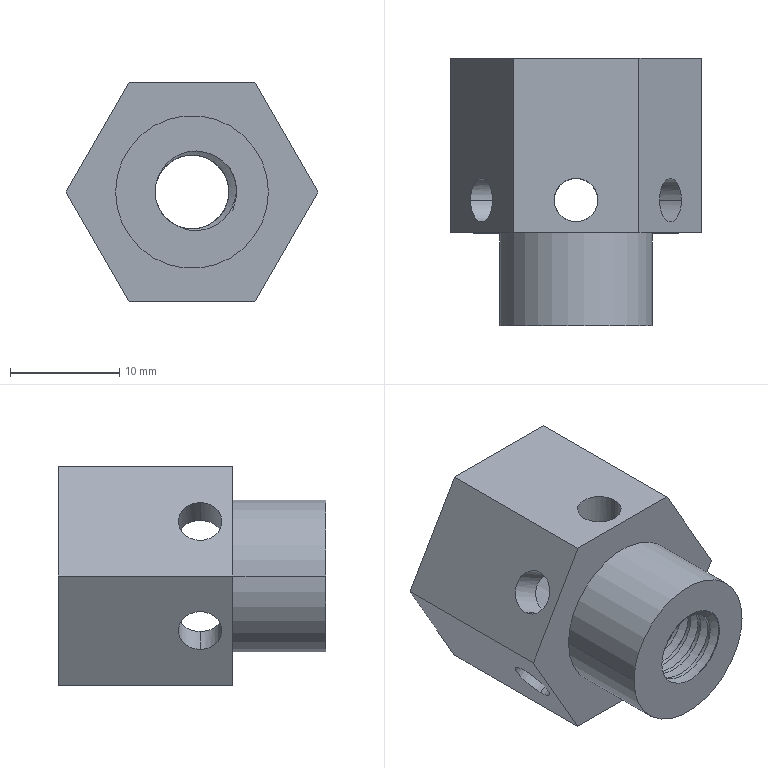Part | SolidWorks | features BaseBody 2 | 2 solids | 57 faces | box 23.094 x 24.5 x 20 mm | volume 3796 mm3 | cylinder 45 | plane 10 | spline 2 | commonest cylinder face diameters 8.17 x14 6.779 x13 4 x12 14 x4 6.78 x2